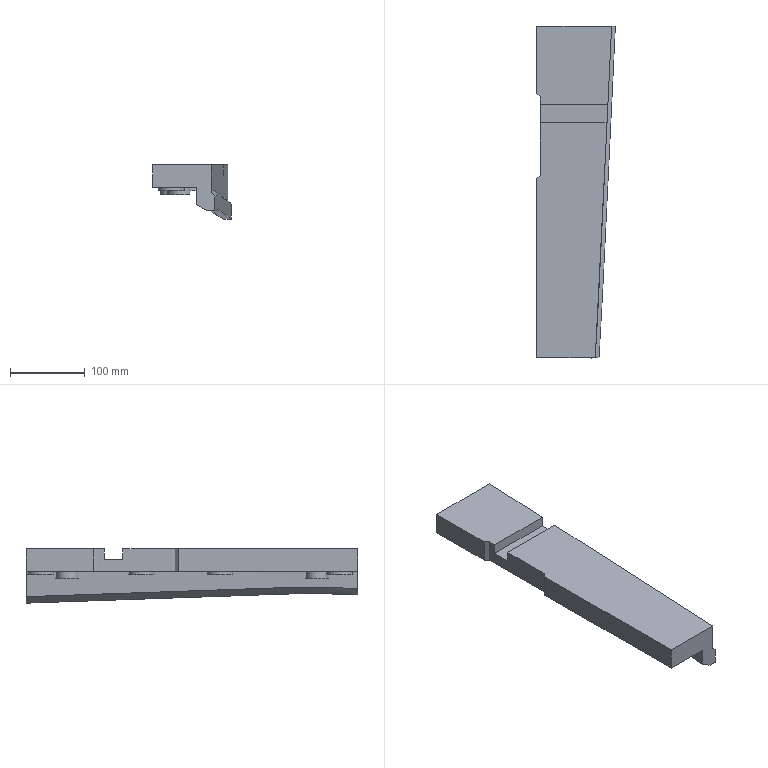Part | NX | features solid 2 | 1 solid | 31 faces | box 105.435 x 445 x 72.8 mm | volume 1519826 mm3 | plane 19 | cylinder 6 | spline 6 | commonest cylinder face diameters 35 x4 30 x2